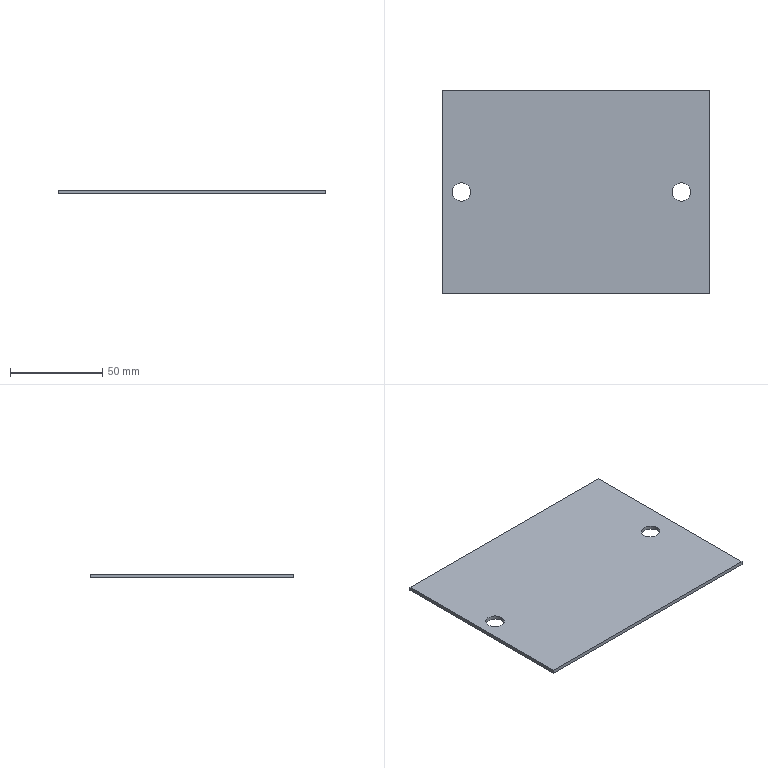Part | STEP file | 1 solid | 10 faces | box 144 x 110 x 2 mm | volume 31366 mm3 | plane 6 | cylinder 4 | commonest cylinder face diameters 10 x4
STEP:
#1=CARTESIAN_POINT('',(0.,0.,0.));
#2=DIRECTION('',(0.,0.,1.));
#3=DIRECTION('',(1.,0.,0.));
#4=AXIS2_PLACEMENT_3D('',#1,#2,#3);
#5=CARTESIAN_POINT('',(31.918,33.653,2.));
#6=VERTEX_POINT('',#5);
#7=CARTESIAN_POINT('',(31.918,33.653,0.));
#8=VERTEX_POINT('',#7);
#9=CARTESIAN_POINT('',(31.918,33.653,2.));
#10=DIRECTION('',(0.,0.,-1.));
#11=VECTOR('',#10,1.);
#12=LINE('',#9,#11);
#13=CARTESIAN_POINT('',(36.918,33.653,2.));
#14=DIRECTION('',(0.,0.,-1.));
#15=DIRECTION('',(-1.,0.,0.));
#16=AXIS2_PLACEMENT_3D('',#13,#14,#15);
#17=CYLINDRICAL_SURFACE('',#16,5.);
#18=CARTESIAN_POINT('',(6.283,0.));
#19=DIRECTION('',(0.,1.));
#20=VECTOR('',#19,1.);
#21=LINE('',#18,#20);
#22=(GEOMETRIC_REPRESENTATION_CONTEXT(2)PARAMETRIC_REPRESENTATION_CONTEXT()REPRESENTATION_CONTEXT('',''));
#23=DEFINITIONAL_REPRESENTATION('',(#21),#22);
#24=PCURVE('',#17,#23);
#25=CARTESIAN_POINT('',(36.918,33.653,2.));
#26=DIRECTION('',(0.,0.,-1.));
#27=DIRECTION('',(-1.,0.,0.));
#28=AXIS2_PLACEMENT_3D('',#25,#26,#27);
#29=CYLINDRICAL_SURFACE('',#28,5.);
#30=CARTESIAN_POINT('',(0.,0.));
#31=DIRECTION('',(0.,1.));
#32=VECTOR('',#31,1.);
#33=LINE('',#30,#32);
#34=(GEOMETRIC_REPRESENTATION_CONTEXT(2)PARAMETRIC_REPRESENTATION_CONTEXT()REPRESENTATION_CONTEXT('',''));
#35=DEFINITIONAL_REPRESENTATION('',(#33),#34);
#36=PCURVE('',#29,#35);
#37=SURFACE_CURVE('',#12,(#24,#36),.PCURVE_S1.);
#38=EDGE_CURVE('',#6,#8,#37,.T.);
#39=ORIENTED_EDGE('',*,*,#38,.T.);
#40=CARTESIAN_POINT('',(41.918,33.653,0.));
#41=VERTEX_POINT('',#40);
#42=CARTESIAN_POINT('',(36.918,33.653,0.));
#43=DIRECTION('',(0.,0.,-1.));
#44=DIRECTION('',(-1.,0.,0.));
#45=AXIS2_PLACEMENT_3D('',#42,#43,#44);
#46=CIRCLE('',#45,5.);
#47=CARTESIAN_POINT('',(0.,2.));
#48=DIRECTION('',(1.,0.));
#49=VECTOR('',#48,1.);
#50=LINE('',#47,#49);
#51=(GEOMETRIC_REPRESENTATION_CONTEXT(2)PARAMETRIC_REPRESENTATION_CONTEXT()REPRESENTATION_CONTEXT('',''));
#52=DEFINITIONAL_REPRESENTATION('',(#50),#51);
#53=PCURVE('',#17,#52);
#54=CARTESIAN_POINT('',(-20.082,33.653,0.));
#55=DIRECTION('',(0.,0.,1.));
#56=DIRECTION('',(1.,0.,0.));
#57=AXIS2_PLACEMENT_3D('',#54,#55,#56);
#58=PLANE('',#57);
#59=CARTESIAN_POINT('',(52.,0.));
#60=CARTESIAN_POINT('',(52.,8.66));
#61=CARTESIAN_POINT('',(59.5,4.33));
#62=CARTESIAN_POINT('',(67.,0.));
#63=CARTESIAN_POINT('',(59.5,-4.33));
#64=CARTESIAN_POINT('',(52.,-8.66));
#65=CARTESIAN_POINT('',(52.,0.));
#66=(BOUNDED_CURVE()B_SPLINE_CURVE(2,(#59,#60,#61,#62,#63,#64,#65),.UNSPECIFIED.,.T.,.F.)B_SPLINE_CURVE_WITH_KNOTS((1,2,2,2,2,1),(-2.094,0.,2.094,4.189,6.283,8.378),.UNSPECIFIED.)CURVE()GEOMETRIC_REPRESENTATION_ITEM()RATIONAL_B_SPLINE_CURVE((1.,0.5,1.,0.5,1.,0.5,1.))REPRESENTATION_ITEM(''));
#67=(GEOMETRIC_REPRESENTATION_CONTEXT(2)PARAMETRIC_REPRESENTATION_CONTEXT()REPRESENTATION_CONTEXT('',''));
#68=DEFINITIONAL_REPRESENTATION('',(#66),#67);
#69=PCURVE('',#58,#68);
#70=SURFACE_CURVE('',#46,(#53,#69),.PCURVE_S1.);
#71=EDGE_CURVE('',#41,#8,#70,.T.);
#72=ORIENTED_EDGE('',*,*,#71,.F.);
#73=CARTESIAN_POINT('',(41.918,33.653,2.));
#74=VERTEX_POINT('',#73);
#75=CARTESIAN_POINT('',(41.918,33.653,2.));
#76=DIRECTION('',(0.,0.,-1.));
#77=VECTOR('',#76,1.);
#78=LINE('',#75,#77);
#79=CARTESIAN_POINT('',(3.142,0.));
#80=DIRECTION('',(0.,1.));
#81=VECTOR('',#80,1.);
#82=LINE('',#79,#81);
#83=(GEOMETRIC_REPRESENTATION_CONTEXT(2)PARAMETRIC_REPRESENTATION_CONTEXT()REPRESENTATION_CONTEXT('',''));
#84=DEFINITIONAL_REPRESENTATION('',(#82),#83);
#85=PCURVE('',#17,#84);
#86=CARTESIAN_POINT('',(3.142,0.));
#87=DIRECTION('',(0.,1.));
#88=VECTOR('',#87,1.);
#89=LINE('',#86,#88);
#90=(GEOMETRIC_REPRESENTATION_CONTEXT(2)PARAMETRIC_REPRESENTATION_CONTEXT()REPRESENTATION_CONTEXT('',''));
#91=DEFINITIONAL_REPRESENTATION('',(#89),#90);
#92=PCURVE('',#29,#91);
#93=SURFACE_CURVE('',#78,(#85,#92),.PCURVE_S1.);
#94=EDGE_CURVE('',#74,#41,#93,.T.);
#95=ORIENTED_EDGE('',*,*,#94,.F.);
#96=CARTESIAN_POINT('',(36.918,33.653,2.));
#97=DIRECTION('',(0.,0.,-1.));
#98=DIRECTION('',(-1.,0.,0.));
#99=AXIS2_PLACEMENT_3D('',#96,#97,#98);
#100=CIRCLE('',#99,5.);
#101=CARTESIAN_POINT('',(0.,0.));
#102=DIRECTION('',(1.,0.));
#103=VECTOR('',#102,1.);
#104=LINE('',#101,#103);
#105=(GEOMETRIC_REPRESENTATION_CONTEXT(2)PARAMETRIC_REPRESENTATION_CONTEXT()REPRESENTATION_CONTEXT('',''));
#106=DEFINITIONAL_REPRESENTATION('',(#104),#105);
#107=PCURVE('',#17,#106);
#108=CARTESIAN_POINT('',(-20.082,33.653,2.));
#109=DIRECTION('',(0.,0.,1.));
#110=DIRECTION('',(1.,0.,0.));
#111=AXIS2_PLACEMENT_3D('',#108,#109,#110);
#112=PLANE('',#111);
#113=CARTESIAN_POINT('',(52.,0.));
#114=CARTESIAN_POINT('',(52.,8.66));
#115=CARTESIAN_POINT('',(59.5,4.33));
#116=CARTESIAN_POINT('',(67.,0.));
#117=CARTESIAN_POINT('',(59.5,-4.33));
#118=CARTESIAN_POINT('',(52.,-8.66));
#119=CARTESIAN_POINT('',(52.,0.));
#120=(BOUNDED_CURVE()B_SPLINE_CURVE(2,(#113,#114,#115,#116,#117,#118,#119),.UNSPECIFIED.,.T.,.F.)B_SPLINE_CURVE_WITH_KNOTS((1,2,2,2,2,1),(-2.094,0.,2.094,4.189,6.283,8.378),.UNSPECIFIED.)CURVE()GEOMETRIC_REPRESENTATION_ITEM()RATIONAL_B_SPLINE_CURVE((1.,0.5,1.,0.5,1.,0.5,1.))REPRESENTATION_ITEM(''));
#121=(GEOMETRIC_REPRESENTATION_CONTEXT(2)PARAMETRIC_REPRESENTATION_CONTEXT()REPRESENTATION_CONTEXT('',''));
#122=DEFINITIONAL_REPRESENTATION('',(#120),#121);
#123=PCURVE('',#112,#122);
#124=SURFACE_CURVE('',#100,(#107,#123),.PCURVE_S1.);
#125=EDGE_CURVE('',#74,#6,#124,.T.);
#126=ORIENTED_EDGE('',*,*,#125,.T.);
#127=EDGE_LOOP('',(#39,#72,#95,#126));
#128=FACE_BOUND('',#127,.F.);
#129=ADVANCED_FACE('',(#128),#17,.F.);
#130=CARTESIAN_POINT('',(-87.082,33.653,2.));
#131=VERTEX_POINT('',#130);
#132=CARTESIAN_POINT('',(-87.082,33.653,0.));
#133=VERTEX_POINT('',#132);
#134=CARTESIAN_POINT('',(-87.082,33.653,2.));
#135=DIRECTION('',(0.,0.,-1.));
#136=VECTOR('',#135,1.);
#137=LINE('',#134,#136);
#138=CARTESIAN_POINT('',(-82.082,33.653,2.));
#139=DIRECTION('',(0.,0.,-1.));
#140=DIRECTION('',(-1.,0.,0.));
#141=AXIS2_PLACEMENT_3D('',#138,#139,#140);
#142=CYLINDRICAL_SURFACE('',#141,5.);
#143=CARTESIAN_POINT('',(6.283,0.));
#144=DIRECTION('',(0.,1.));
#145=VECTOR('',#144,1.);
#146=LINE('',#143,#145);
#147=(GEOMETRIC_REPRESENTATION_CONTEXT(2)PARAMETRIC_REPRESENTATION_CONTEXT()REPRESENTATION_CONTEXT('',''));
#148=DEFINITIONAL_REPRESENTATION('',(#146),#147);
#149=PCURVE('',#142,#148);
#150=CARTESIAN_POINT('',(-82.082,33.653,2.));
#151=DIRECTION('',(0.,0.,-1.));
#152=DIRECTION('',(-1.,0.,0.));
#153=AXIS2_PLACEMENT_3D('',#150,#151,#152);
#154=CYLINDRICAL_SURFACE('',#153,5.);
#155=CARTESIAN_POINT('',(0.,0.));
#156=DIRECTION('',(0.,1.));
#157=VECTOR('',#156,1.);
#158=LINE('',#155,#157);
#159=(GEOMETRIC_REPRESENTATION_CONTEXT(2)PARAMETRIC_REPRESENTATION_CONTEXT()REPRESENTATION_CONTEXT('',''));
#160=DEFINITIONAL_REPRESENTATION('',(#158),#159);
#161=PCURVE('',#154,#160);
#162=SURFACE_CURVE('',#137,(#149,#161),.PCURVE_S1.);
#163=EDGE_CURVE('',#131,#133,#162,.T.);
#164=ORIENTED_EDGE('',*,*,#163,.T.);
#165=CARTESIAN_POINT('',(-77.082,33.653,0.));
#166=VERTEX_POINT('',#165);
#167=CARTESIAN_POINT('',(-82.082,33.653,0.));
#168=DIRECTION('',(0.,0.,-1.));
#169=DIRECTION('',(-1.,0.,0.));
#170=AXIS2_PLACEMENT_3D('',#167,#168,#169);
#171=CIRCLE('',#170,5.);
#172=CARTESIAN_POINT('',(0.,2.));
#173=DIRECTION('',(1.,0.));
#174=VECTOR('',#173,1.);
#175=LINE('',#172,#174);
#176=(GEOMETRIC_REPRESENTATION_CONTEXT(2)PARAMETRIC_REPRESENTATION_CONTEXT()REPRESENTATION_CONTEXT('',''));
#177=DEFINITIONAL_REPRESENTATION('',(#175),#176);
#178=PCURVE('',#142,#177);
#179=CARTESIAN_POINT('',(-67.,0.));
#180=CARTESIAN_POINT('',(-67.,8.66));
#181=CARTESIAN_POINT('',(-59.5,4.33));
#182=CARTESIAN_POINT('',(-52.,0.));
#183=CARTESIAN_POINT('',(-59.5,-4.33));
#184=CARTESIAN_POINT('',(-67.,-8.66));
#185=CARTESIAN_POINT('',(-67.,0.));
#186=(BOUNDED_CURVE()B_SPLINE_CURVE(2,(#179,#180,#181,#182,#183,#184,#185),.UNSPECIFIED.,.T.,.F.)B_SPLINE_CURVE_WITH_KNOTS((1,2,2,2,2,1),(-2.094,0.,2.094,4.189,6.283,8.378),.UNSPECIFIED.)CURVE()GEOMETRIC_REPRESENTATION_ITEM()RATIONAL_B_SPLINE_CURVE((1.,0.5,1.,0.5,1.,0.5,1.))REPRESENTATION_ITEM(''));
#187=(GEOMETRIC_REPRESENTATION_CONTEXT(2)PARAMETRIC_REPRESENTATION_CONTEXT()REPRESENTATION_CONTEXT('',''));
#188=DEFINITIONAL_REPRESENTATION('',(#186),#187);
#189=PCURVE('',#58,#188);
#190=SURFACE_CURVE('',#171,(#178,#189),.PCURVE_S1.);
#191=EDGE_CURVE('',#166,#133,#190,.T.);
#192=ORIENTED_EDGE('',*,*,#191,.F.);
#193=CARTESIAN_POINT('',(-77.082,33.653,2.));
#194=VERTEX_POINT('',#193);
#195=CARTESIAN_POINT('',(-77.082,33.653,2.));
#196=DIRECTION('',(0.,0.,-1.));
#197=VECTOR('',#196,1.);
#198=LINE('',#195,#197);
#199=CARTESIAN_POINT('',(3.142,0.));
#200=DIRECTION('',(0.,1.));
#201=VECTOR('',#200,1.);
#202=LINE('',#199,#201);
#203=(GEOMETRIC_REPRESENTATION_CONTEXT(2)PARAMETRIC_REPRESENTATION_CONTEXT()REPRESENTATION_CONTEXT('',''));
#204=DEFINITIONAL_REPRESENTATION('',(#202),#203);
#205=PCURVE('',#142,#204);
#206=CARTESIAN_POINT('',(3.142,0.));
#207=DIRECTION('',(0.,1.));
#208=VECTOR('',#207,1.);
#209=LINE('',#206,#208);
#210=(GEOMETRIC_REPRESENTATION_CONTEXT(2)PARAMETRIC_REPRESENTATION_CONTEXT()REPRESENTATION_CONTEXT('',''));
#211=DEFINITIONAL_REPRESENTATION('',(#209),#210);
#212=PCURVE('',#154,#211);
#213=SURFACE_CURVE('',#198,(#205,#212),.PCURVE_S1.);
#214=EDGE_CURVE('',#194,#166,#213,.T.);
#215=ORIENTED_EDGE('',*,*,#214,.F.);
#216=CARTESIAN_POINT('',(-82.082,33.653,2.));
#217=DIRECTION('',(0.,0.,-1.));
#218=DIRECTION('',(-1.,0.,0.));
#219=AXIS2_PLACEMENT_3D('',#216,#217,#218);
#220=CIRCLE('',#219,5.);
#221=CARTESIAN_POINT('',(0.,0.));
#222=DIRECTION('',(1.,0.));
#223=VECTOR('',#222,1.);
#224=LINE('',#221,#223);
#225=(GEOMETRIC_REPRESENTATION_CONTEXT(2)PARAMETRIC_REPRESENTATION_CONTEXT()REPRESENTATION_CONTEXT('',''));
#226=DEFINITIONAL_REPRESENTATION('',(#224),#225);
#227=PCURVE('',#142,#226);
#228=CARTESIAN_POINT('',(-67.,0.));
#229=CARTESIAN_POINT('',(-67.,8.66));
#230=CARTESIAN_POINT('',(-59.5,4.33));
#231=CARTESIAN_POINT('',(-52.,0.));
#232=CARTESIAN_POINT('',(-59.5,-4.33));
#233=CARTESIAN_POINT('',(-67.,-8.66));
#234=CARTESIAN_POINT('',(-67.,0.));
#235=(BOUNDED_CURVE()B_SPLINE_CURVE(2,(#228,#229,#230,#231,#232,#233,#234),.UNSPECIFIED.,.T.,.F.)B_SPLINE_CURVE_WITH_KNOTS((1,2,2,2,2,1),(-2.094,0.,2.094,4.189,6.283,8.378),.UNSPECIFIED.)CURVE()GEOMETRIC_REPRESENTATION_ITEM()RATIONAL_B_SPLINE_CURVE((1.,0.5,1.,0.5,1.,0.5,1.))REPRESENTATION_ITEM(''));
#236=(GEOMETRIC_REPRESENTATION_CONTEXT(2)PARAMETRIC_REPRESENTATION_CONTEXT()REPRESENTATION_CONTEXT('',''));
#237=DEFINITIONAL_REPRESENTATION('',(#235),#236);
#238=PCURVE('',#112,#237);
#239=SURFACE_CURVE('',#220,(#227,#238),.PCURVE_S1.);
#240=EDGE_CURVE('',#194,#131,#239,.T.);
#241=ORIENTED_EDGE('',*,*,#240,.T.);
#242=EDGE_LOOP('',(#164,#192,#215,#241));
#243=FACE_BOUND('',#242,.F.);
#244=ADVANCED_FACE('',(#243),#142,.F.);
#245=CARTESIAN_POINT('',(51.918,-21.347,0.));
#246=VERTEX_POINT('',#245);
#247=CARTESIAN_POINT('',(51.918,88.653,0.));
#248=VERTEX_POINT('',#247);
#249=CARTESIAN_POINT('',(51.918,33.653,0.));
#250=DIRECTION('',(0.,1.,0.));
#251=VECTOR('',#250,1.);
#252=LINE('',#249,#251);
#253=CARTESIAN_POINT('',(72.,0.));
#254=DIRECTION('',(0.,1.));
#255=VECTOR('',#254,1.);
#256=LINE('',#253,#255);
#257=(GEOMETRIC_REPRESENTATION_CONTEXT(2)PARAMETRIC_REPRESENTATION_CONTEXT()REPRESENTATION_CONTEXT('',''));
#258=DEFINITIONAL_REPRESENTATION('',(#256),#257);
#259=PCURVE('',#58,#258);
#260=CARTESIAN_POINT('',(51.918,-21.347,0.));
#261=DIRECTION('',(1.,0.,0.));
#262=DIRECTION('',(0.,1.,0.));
#263=AXIS2_PLACEMENT_3D('',#260,#261,#262);
#264=PLANE('',#263);
#265=CARTESIAN_POINT('',(55.,0.));
#266=DIRECTION('',(1.,0.));
#267=VECTOR('',#266,1.);
#268=LINE('',#265,#267);
#269=(GEOMETRIC_REPRESENTATION_CONTEXT(2)PARAMETRIC_REPRESENTATION_CONTEXT()REPRESENTATION_CONTEXT('',''));
#270=DEFINITIONAL_REPRESENTATION('',(#268),#269);
#271=PCURVE('',#264,#270);
#272=SURFACE_CURVE('',#252,(#259,#271),.PCURVE_S1.);
#273=EDGE_CURVE('',#246,#248,#272,.T.);
#274=ORIENTED_EDGE('',*,*,#273,.F.);
#275=CARTESIAN_POINT('',(-92.082,-21.347,0.));
#276=VERTEX_POINT('',#275);
#277=CARTESIAN_POINT('',(-20.082,-21.347,0.));
#278=DIRECTION('',(1.,0.,0.));
#279=VECTOR('',#278,1.);
#280=LINE('',#277,#279);
#281=CARTESIAN_POINT('',(0.,-55.));
#282=DIRECTION('',(1.,0.));
#283=VECTOR('',#282,1.);
#284=LINE('',#281,#283);
#285=(GEOMETRIC_REPRESENTATION_CONTEXT(2)PARAMETRIC_REPRESENTATION_CONTEXT()REPRESENTATION_CONTEXT('',''));
#286=DEFINITIONAL_REPRESENTATION('',(#284),#285);
#287=PCURVE('',#58,#286);
#288=CARTESIAN_POINT('',(-92.082,-21.347,0.));
#289=DIRECTION('',(0.,-1.,0.));
#290=DIRECTION('',(1.,0.,0.));
#291=AXIS2_PLACEMENT_3D('',#288,#289,#290);
#292=PLANE('',#291);
#293=CARTESIAN_POINT('',(72.,0.));
#294=DIRECTION('',(1.,0.));
#295=VECTOR('',#294,1.);
#296=LINE('',#293,#295);
#297=(GEOMETRIC_REPRESENTATION_CONTEXT(2)PARAMETRIC_REPRESENTATION_CONTEXT()REPRESENTATION_CONTEXT('',''));
#298=DEFINITIONAL_REPRESENTATION('',(#296),#297);
#299=PCURVE('',#292,#298);
#300=SURFACE_CURVE('',#280,(#287,#299),.PCURVE_S1.);
#301=EDGE_CURVE('',#276,#246,#300,.T.);
#302=ORIENTED_EDGE('',*,*,#301,.F.);
#303=CARTESIAN_POINT('',(-92.082,88.653,0.));
#304=VERTEX_POINT('',#303);
#305=CARTESIAN_POINT('',(-92.082,33.653,0.));
#306=DIRECTION('',(0.,-1.,0.));
#307=VECTOR('',#306,1.);
#308=LINE('',#305,#307);
#309=CARTESIAN_POINT('',(-72.,0.));
#310=DIRECTION('',(0.,-1.));
#311=VECTOR('',#310,1.);
#312=LINE('',#309,#311);
#313=(GEOMETRIC_REPRESENTATION_CONTEXT(2)PARAMETRIC_REPRESENTATION_CONTEXT()REPRESENTATION_CONTEXT('',''));
#314=DEFINITIONAL_REPRESENTATION('',(#312),#313);
#315=PCURVE('',#58,#314);
#316=CARTESIAN_POINT('',(-92.082,88.653,0.));
#317=DIRECTION('',(-1.,0.,0.));
#318=DIRECTION('',(0.,-1.,0.));
#319=AXIS2_PLACEMENT_3D('',#316,#317,#318);
#320=PLANE('',#319);
#321=CARTESIAN_POINT('',(55.,0.));
#322=DIRECTION('',(1.,0.));
#323=VECTOR('',#322,1.);
#324=LINE('',#321,#323);
#325=(GEOMETRIC_REPRESENTATION_CONTEXT(2)PARAMETRIC_REPRESENTATION_CONTEXT()REPRESENTATION_CONTEXT('',''));
#326=DEFINITIONAL_REPRESENTATION('',(#324),#325);
#327=PCURVE('',#320,#326);
#328=SURFACE_CURVE('',#308,(#315,#327),.PCURVE_S1.);
#329=EDGE_CURVE('',#304,#276,#328,.T.);
#330=ORIENTED_EDGE('',*,*,#329,.F.);
#331=CARTESIAN_POINT('',(-20.082,88.653,0.));
#332=DIRECTION('',(-1.,0.,0.));
#333=VECTOR('',#332,1.);
#334=LINE('',#331,#333);
#335=CARTESIAN_POINT('',(0.,55.));
#336=DIRECTION('',(-1.,0.));
#337=VECTOR('',#336,1.);
#338=LINE('',#335,#337);
#339=(GEOMETRIC_REPRESENTATION_CONTEXT(2)PARAMETRIC_REPRESENTATION_CONTEXT()REPRESENTATION_CONTEXT('',''));
#340=DEFINITIONAL_REPRESENTATION('',(#338),#339);
#341=PCURVE('',#58,#340);
#342=CARTESIAN_POINT('',(51.918,88.653,0.));
#343=DIRECTION('',(0.,1.,0.));
#344=DIRECTION('',(0.,0.,1.));
#345=AXIS2_PLACEMENT_3D('',#342,#343,#344);
#346=PLANE('',#345);
#347=CARTESIAN_POINT('',(0.,-72.));
#348=DIRECTION('',(0.,-1.));
#349=VECTOR('',#348,1.);
#350=LINE('',#347,#349);
#351=(GEOMETRIC_REPRESENTATION_CONTEXT(2)PARAMETRIC_REPRESENTATION_CONTEXT()REPRESENTATION_CONTEXT('',''));
#352=DEFINITIONAL_REPRESENTATION('',(#350),#351);
#353=PCURVE('',#346,#352);
#354=SURFACE_CURVE('',#334,(#341,#353),.PCURVE_S1.);
#355=EDGE_CURVE('',#248,#304,#354,.T.);
#356=ORIENTED_EDGE('',*,*,#355,.F.);
#357=EDGE_LOOP('',(#274,#302,#330,#356));
#358=FACE_BOUND('',#357,.T.);
#359=CARTESIAN_POINT('',(36.918,33.653,0.));
#360=DIRECTION('',(0.,0.,-1.));
#361=DIRECTION('',(-1.,0.,0.));
#362=AXIS2_PLACEMENT_3D('',#359,#360,#361);
#363=CIRCLE('',#362,5.);
#364=CARTESIAN_POINT('',(52.,0.));
#365=CARTESIAN_POINT('',(52.,8.66));
#366=CARTESIAN_POINT('',(59.5,4.33));
#367=CARTESIAN_POINT('',(67.,0.));
#368=CARTESIAN_POINT('',(59.5,-4.33));
#369=CARTESIAN_POINT('',(52.,-8.66));
#370=CARTESIAN_POINT('',(52.,0.));
#371=(BOUNDED_CURVE()B_SPLINE_CURVE(2,(#364,#365,#366,#367,#368,#369,#370),.UNSPECIFIED.,.T.,.F.)B_SPLINE_CURVE_WITH_KNOTS((1,2,2,2,2,1),(-2.094,0.,2.094,4.189,6.283,8.378),.UNSPECIFIED.)CURVE()GEOMETRIC_REPRESENTATION_ITEM()RATIONAL_B_SPLINE_CURVE((1.,0.5,1.,0.5,1.,0.5,1.))REPRESENTATION_ITEM(''));
#372=(GEOMETRIC_REPRESENTATION_CONTEXT(2)PARAMETRIC_REPRESENTATION_CONTEXT()REPRESENTATION_CONTEXT('',''));
#373=DEFINITIONAL_REPRESENTATION('',(#371),#372);
#374=PCURVE('',#58,#373);
#375=CARTESIAN_POINT('',(0.,2.));
#376=DIRECTION('',(1.,0.));
#377=VECTOR('',#376,1.);
#378=LINE('',#375,#377);
#379=(GEOMETRIC_REPRESENTATION_CONTEXT(2)PARAMETRIC_REPRESENTATION_CONTEXT()REPRESENTATION_CONTEXT('',''));
#380=DEFINITIONAL_REPRESENTATION('',(#378),#379);
#381=PCURVE('',#29,#380);
#382=SURFACE_CURVE('',#363,(#374,#381),.PCURVE_S1.);
#383=EDGE_CURVE('',#8,#41,#382,.T.);
#384=ORIENTED_EDGE('',*,*,#383,.F.);
#385=ORIENTED_EDGE('',*,*,#71,.F.);
#386=EDGE_LOOP('',(#384,#385));
#387=FACE_BOUND('',#386,.T.);
#388=CARTESIAN_POINT('',(-82.082,33.653,0.));
#389=DIRECTION('',(0.,0.,-1.));
#390=DIRECTION('',(-1.,0.,0.));
#391=AXIS2_PLACEMENT_3D('',#388,#389,#390);
#392=CIRCLE('',#391,5.);
#393=CARTESIAN_POINT('',(-67.,0.));
#394=CARTESIAN_POINT('',(-67.,8.66));
#395=CARTESIAN_POINT('',(-59.5,4.33));
#396=CARTESIAN_POINT('',(-52.,0.));
#397=CARTESIAN_POINT('',(-59.5,-4.33));
#398=CARTESIAN_POINT('',(-67.,-8.66));
#399=CARTESIAN_POINT('',(-67.,0.));
#400=(BOUNDED_CURVE()B_SPLINE_CURVE(2,(#393,#394,#395,#396,#397,#398,#399),.UNSPECIFIED.,.T.,.F.)B_SPLINE_CURVE_WITH_KNOTS((1,2,2,2,2,1),(-2.094,0.,2.094,4.189,6.283,8.378),.UNSPECIFIED.)CURVE()GEOMETRIC_REPRESENTATION_ITEM()RATIONAL_B_SPLINE_CURVE((1.,0.5,1.,0.5,1.,0.5,1.))REPRESENTATION_ITEM(''));
#401=(GEOMETRIC_REPRESENTATION_CONTEXT(2)PARAMETRIC_REPRESENTATION_CONTEXT()REPRESENTATION_CONTEXT('',''));
#402=DEFINITIONAL_REPRESENTATION('',(#400),#401);
#403=PCURVE('',#58,#402);
#404=CARTESIAN_POINT('',(0.,2.));
#405=DIRECTION('',(1.,0.));
#406=VECTOR('',#405,1.);
#407=LINE('',#404,#406);
#408=(GEOMETRIC_REPRESENTATION_CONTEXT(2)PARAMETRIC_REPRESENTATION_CONTEXT()REPRESENTATION_CONTEXT('',''));
#409=DEFINITIONAL_REPRESENTATION('',(#407),#408);
#410=PCURVE('',#154,#409);
#411=SURFACE_CURVE('',#392,(#403,#410),.PCURVE_S1.);
#412=EDGE_CURVE('',#133,#166,#411,.T.);
#413=ORIENTED_EDGE('',*,*,#412,.F.);
#414=ORIENTED_EDGE('',*,*,#191,.F.);
#415=EDGE_LOOP('',(#413,#414));
#416=FACE_BOUND('',#415,.T.);
#417=ADVANCED_FACE('',(#358,#387,#416),#58,.F.);
#418=CARTESIAN_POINT('',(-92.082,88.653,2.));
#419=VERTEX_POINT('',#418);
#420=CARTESIAN_POINT('',(51.918,88.653,2.));
#421=VERTEX_POINT('',#420);
#422=CARTESIAN_POINT('',(51.918,88.653,2.));
#423=DIRECTION('',(1.,0.,0.));
#424=VECTOR('',#423,1.);
#425=LINE('',#422,#424);
#426=CARTESIAN_POINT('',(2.,0.));
#427=DIRECTION('',(0.,1.));
#428=VECTOR('',#427,1.);
#429=LINE('',#426,#428);
#430=(GEOMETRIC_REPRESENTATION_CONTEXT(2)PARAMETRIC_REPRESENTATION_CONTEXT()REPRESENTATION_CONTEXT('',''));
#431=DEFINITIONAL_REPRESENTATION('',(#429),#430);
#432=PCURVE('',#346,#431);
#433=CARTESIAN_POINT('',(72.,55.));
#434=DIRECTION('',(1.,0.));
#435=VECTOR('',#434,1.);
#436=LINE('',#433,#435);
#437=(GEOMETRIC_REPRESENTATION_CONTEXT(2)PARAMETRIC_REPRESENTATION_CONTEXT()REPRESENTATION_CONTEXT('',''));
#438=DEFINITIONAL_REPRESENTATION('',(#436),#437);
#439=PCURVE('',#112,#438);
#440=SURFACE_CURVE('',#425,(#432,#439),.PCURVE_S1.);
#441=EDGE_CURVE('',#419,#421,#440,.T.);
#442=ORIENTED_EDGE('',*,*,#441,.T.);
#443=CARTESIAN_POINT('',(51.918,88.653,0.));
#444=DIRECTION('',(0.,0.,-1.));
#445=VECTOR('',#444,1.);
#446=LINE('',#443,#445);
#447=CARTESIAN_POINT('',(0.,0.));
#448=DIRECTION('',(-1.,0.));
#449=VECTOR('',#448,1.);
#450=LINE('',#447,#449);
#451=(GEOMETRIC_REPRESENTATION_CONTEXT(2)PARAMETRIC_REPRESENTATION_CONTEXT()REPRESENTATION_CONTEXT('',''));
#452=DEFINITIONAL_REPRESENTATION('',(#450),#451);
#453=PCURVE('',#346,#452);
#454=CARTESIAN_POINT('',(110.,0.));
#455=DIRECTION('',(0.,-1.));
#456=VECTOR('',#455,1.);
#457=LINE('',#454,#456);
#458=(GEOMETRIC_REPRESENTATION_CONTEXT(2)PARAMETRIC_REPRESENTATION_CONTEXT()REPRESENTATION_CONTEXT('',''));
#459=DEFINITIONAL_REPRESENTATION('',(#457),#458);
#460=PCURVE('',#264,#459);
#461=SURFACE_CURVE('',#446,(#453,#460),.PCURVE_S1.);
#462=EDGE_CURVE('',#421,#248,#461,.T.);
#463=ORIENTED_EDGE('',*,*,#462,.T.);
#464=ORIENTED_EDGE('',*,*,#355,.T.);
#465=CARTESIAN_POINT('',(-92.082,88.653,0.));
#466=DIRECTION('',(0.,0.,1.));
#467=VECTOR('',#466,1.);
#468=LINE('',#465,#467);
#469=CARTESIAN_POINT('',(0.,-144.));
#470=DIRECTION('',(1.,0.));
#471=VECTOR('',#470,1.);
#472=LINE('',#469,#471);
#473=(GEOMETRIC_REPRESENTATION_CONTEXT(2)PARAMETRIC_REPRESENTATION_CONTEXT()REPRESENTATION_CONTEXT('',''));
#474=DEFINITIONAL_REPRESENTATION('',(#472),#473);
#475=PCURVE('',#346,#474);
#476=CARTESIAN_POINT('',(0.,0.));
#477=DIRECTION('',(0.,1.));
#478=VECTOR('',#477,1.);
#479=LINE('',#476,#478);
#480=(GEOMETRIC_REPRESENTATION_CONTEXT(2)PARAMETRIC_REPRESENTATION_CONTEXT()REPRESENTATION_CONTEXT('',''));
#481=DEFINITIONAL_REPRESENTATION('',(#479),#480);
#482=PCURVE('',#320,#481);
#483=SURFACE_CURVE('',#468,(#475,#482),.PCURVE_S1.);
#484=EDGE_CURVE('',#304,#419,#483,.T.);
#485=ORIENTED_EDGE('',*,*,#484,.T.);
#486=EDGE_LOOP('',(#442,#463,#464,#485));
#487=FACE_BOUND('',#486,.T.);
#488=ADVANCED_FACE('',(#487),#346,.T.);
#489=CARTESIAN_POINT('',(51.918,-21.347,2.));
#490=VERTEX_POINT('',#489);
#491=CARTESIAN_POINT('',(51.918,-21.347,2.));
#492=DIRECTION('',(0.,-1.,0.));
#493=VECTOR('',#492,1.);
#494=LINE('',#491,#493);
#495=CARTESIAN_POINT('',(0.,2.));
#496=DIRECTION('',(-1.,0.));
#497=VECTOR('',#496,1.);
#498=LINE('',#495,#497);
#499=(GEOMETRIC_REPRESENTATION_CONTEXT(2)PARAMETRIC_REPRESENTATION_CONTEXT()REPRESENTATION_CONTEXT('',''));
#500=DEFINITIONAL_REPRESENTATION('',(#498),#499);
#501=PCURVE('',#264,#500);
#502=CARTESIAN_POINT('',(72.,-55.));
#503=DIRECTION('',(0.,-1.));
#504=VECTOR('',#503,1.);
#505=LINE('',#502,#504);
#506=(GEOMETRIC_REPRESENTATION_CONTEXT(2)PARAMETRIC_REPRESENTATION_CONTEXT()REPRESENTATION_CONTEXT('',''));
#507=DEFINITIONAL_REPRESENTATION('',(#505),#506);
#508=PCURVE('',#112,#507);
#509=SURFACE_CURVE('',#494,(#501,#508),.PCURVE_S1.);
#510=EDGE_CURVE('',#421,#490,#509,.T.);
#511=ORIENTED_EDGE('',*,*,#510,.T.);
#512=CARTESIAN_POINT('',(51.918,-21.347,0.));
#513=DIRECTION('',(0.,0.,-1.));
#514=VECTOR('',#513,1.);
#515=LINE('',#512,#514);
#516=CARTESIAN_POINT('',(0.,0.));
#517=DIRECTION('',(0.,-1.));
#518=VECTOR('',#517,1.);
#519=LINE('',#516,#518);
#520=(GEOMETRIC_REPRESENTATION_CONTEXT(2)PARAMETRIC_REPRESENTATION_CONTEXT()REPRESENTATION_CONTEXT('',''));
#521=DEFINITIONAL_REPRESENTATION('',(#519),#520);
#522=PCURVE('',#264,#521);
#523=CARTESIAN_POINT('',(144.,0.));
#524=DIRECTION('',(0.,-1.));
#525=VECTOR('',#524,1.);
#526=LINE('',#523,#525);
#527=(GEOMETRIC_REPRESENTATION_CONTEXT(2)PARAMETRIC_REPRESENTATION_CONTEXT()REPRESENTATION_CONTEXT('',''));
#528=DEFINITIONAL_REPRESENTATION('',(#526),#527);
#529=PCURVE('',#292,#528);
#530=SURFACE_CURVE('',#515,(#522,#529),.PCURVE_S1.);
#531=EDGE_CURVE('',#490,#246,#530,.T.);
#532=ORIENTED_EDGE('',*,*,#531,.T.);
#533=ORIENTED_EDGE('',*,*,#273,.T.);
#534=ORIENTED_EDGE('',*,*,#462,.F.);
#535=EDGE_LOOP('',(#511,#532,#533,#534));
#536=FACE_BOUND('',#535,.T.);
#537=ADVANCED_FACE('',(#536),#264,.T.);
#538=CARTESIAN_POINT('',(-92.082,-21.347,2.));
#539=VERTEX_POINT('',#538);
#540=CARTESIAN_POINT('',(-92.082,-21.347,2.));
#541=DIRECTION('',(-1.,0.,0.));
#542=VECTOR('',#541,1.);
#543=LINE('',#540,#542);
#544=CARTESIAN_POINT('',(0.,2.));
#545=DIRECTION('',(-1.,0.));
#546=VECTOR('',#545,1.);
#547=LINE('',#544,#546);
#548=(GEOMETRIC_REPRESENTATION_CONTEXT(2)PARAMETRIC_REPRESENTATION_CONTEXT()REPRESENTATION_CONTEXT('',''));
#549=DEFINITIONAL_REPRESENTATION('',(#547),#548);
#550=PCURVE('',#292,#549);
#551=CARTESIAN_POINT('',(-72.,-55.));
#552=DIRECTION('',(-1.,0.));
#553=VECTOR('',#552,1.);
#554=LINE('',#551,#553);
#555=(GEOMETRIC_REPRESENTATION_CONTEXT(2)PARAMETRIC_REPRESENTATION_CONTEXT()REPRESENTATION_CONTEXT('',''));
#556=DEFINITIONAL_REPRESENTATION('',(#554),#555);
#557=PCURVE('',#112,#556);
#558=SURFACE_CURVE('',#543,(#550,#557),.PCURVE_S1.);
#559=EDGE_CURVE('',#490,#539,#558,.T.);
#560=ORIENTED_EDGE('',*,*,#559,.T.);
#561=CARTESIAN_POINT('',(-92.082,-21.347,0.));
#562=DIRECTION('',(0.,0.,-1.));
#563=VECTOR('',#562,1.);
#564=LINE('',#561,#563);
#565=CARTESIAN_POINT('',(0.,0.));
#566=DIRECTION('',(0.,-1.));
#567=VECTOR('',#566,1.);
#568=LINE('',#565,#567);
#569=(GEOMETRIC_REPRESENTATION_CONTEXT(2)PARAMETRIC_REPRESENTATION_CONTEXT()REPRESENTATION_CONTEXT('',''));
#570=DEFINITIONAL_REPRESENTATION('',(#568),#569);
#571=PCURVE('',#292,#570);
#572=CARTESIAN_POINT('',(110.,0.));
#573=DIRECTION('',(0.,-1.));
#574=VECTOR('',#573,1.);
#575=LINE('',#572,#574);
#576=(GEOMETRIC_REPRESENTATION_CONTEXT(2)PARAMETRIC_REPRESENTATION_CONTEXT()REPRESENTATION_CONTEXT('',''));
#577=DEFINITIONAL_REPRESENTATION('',(#575),#576);
#578=PCURVE('',#320,#577);
#579=SURFACE_CURVE('',#564,(#571,#578),.PCURVE_S1.);
#580=EDGE_CURVE('',#539,#276,#579,.T.);
#581=ORIENTED_EDGE('',*,*,#580,.T.);
#582=ORIENTED_EDGE('',*,*,#301,.T.);
#583=ORIENTED_EDGE('',*,*,#531,.F.);
#584=EDGE_LOOP('',(#560,#581,#582,#583));
#585=FACE_BOUND('',#584,.T.);
#586=ADVANCED_FACE('',(#585),#292,.T.);
#587=CARTESIAN_POINT('',(-92.082,88.653,2.));
#588=DIRECTION('',(0.,1.,0.));
#589=VECTOR('',#588,1.);
#590=LINE('',#587,#589);
#591=CARTESIAN_POINT('',(0.,2.));
#592=DIRECTION('',(-1.,0.));
#593=VECTOR('',#592,1.);
#594=LINE('',#591,#593);
#595=(GEOMETRIC_REPRESENTATION_CONTEXT(2)PARAMETRIC_REPRESENTATION_CONTEXT()REPRESENTATION_CONTEXT('',''));
#596=DEFINITIONAL_REPRESENTATION('',(#594),#595);
#597=PCURVE('',#320,#596);
#598=CARTESIAN_POINT('',(-72.,55.));
#599=DIRECTION('',(0.,1.));
#600=VECTOR('',#599,1.);
#601=LINE('',#598,#600);
#602=(GEOMETRIC_REPRESENTATION_CONTEXT(2)PARAMETRIC_REPRESENTATION_CONTEXT()REPRESENTATION_CONTEXT('',''));
#603=DEFINITIONAL_REPRESENTATION('',(#601),#602);
#604=PCURVE('',#112,#603);
#605=SURFACE_CURVE('',#590,(#597,#604),.PCURVE_S1.);
#606=EDGE_CURVE('',#539,#419,#605,.T.);
#607=ORIENTED_EDGE('',*,*,#606,.T.);
#608=ORIENTED_EDGE('',*,*,#484,.F.);
#609=ORIENTED_EDGE('',*,*,#329,.T.);
#610=ORIENTED_EDGE('',*,*,#580,.F.);
#611=EDGE_LOOP('',(#607,#608,#609,#610));
#612=FACE_BOUND('',#611,.T.);
#613=ADVANCED_FACE('',(#612),#320,.T.);
#614=ORIENTED_EDGE('',*,*,#383,.F.);
#615=ORIENTED_EDGE('',*,*,#38,.F.);
#616=CARTESIAN_POINT('',(36.918,33.653,2.));
#617=DIRECTION('',(0.,0.,-1.));
#618=DIRECTION('',(-1.,0.,0.));
#619=AXIS2_PLACEMENT_3D('',#616,#617,#618);
#620=CIRCLE('',#619,5.);
#621=CARTESIAN_POINT('',(0.,0.));
#622=DIRECTION('',(1.,0.));
#623=VECTOR('',#622,1.);
#624=LINE('',#621,#623);
#625=(GEOMETRIC_REPRESENTATION_CONTEXT(2)PARAMETRIC_REPRESENTATION_CONTEXT()REPRESENTATION_CONTEXT('',''));
#626=DEFINITIONAL_REPRESENTATION('',(#624),#625);
#627=PCURVE('',#29,#626);
#628=CARTESIAN_POINT('',(52.,0.));
#629=CARTESIAN_POINT('',(52.,8.66));
#630=CARTESIAN_POINT('',(59.5,4.33));
#631=CARTESIAN_POINT('',(67.,0.));
#632=CARTESIAN_POINT('',(59.5,-4.33));
#633=CARTESIAN_POINT('',(52.,-8.66));
#634=CARTESIAN_POINT('',(52.,0.));
#635=(BOUNDED_CURVE()B_SPLINE_CURVE(2,(#628,#629,#630,#631,#632,#633,#634),.UNSPECIFIED.,.T.,.F.)B_SPLINE_CURVE_WITH_KNOTS((1,2,2,2,2,1),(-2.094,0.,2.094,4.189,6.283,8.378),.UNSPECIFIED.)CURVE()GEOMETRIC_REPRESENTATION_ITEM()RATIONAL_B_SPLINE_CURVE((1.,0.5,1.,0.5,1.,0.5,1.))REPRESENTATION_ITEM(''));
#636=(GEOMETRIC_REPRESENTATION_CONTEXT(2)PARAMETRIC_REPRESENTATION_CONTEXT()REPRESENTATION_CONTEXT('',''));
#637=DEFINITIONAL_REPRESENTATION('',(#635),#636);
#638=PCURVE('',#112,#637);
#639=SURFACE_CURVE('',#620,(#627,#638),.PCURVE_S1.);
#640=EDGE_CURVE('',#6,#74,#639,.T.);
#641=ORIENTED_EDGE('',*,*,#640,.T.);
#642=ORIENTED_EDGE('',*,*,#94,.T.);
#643=EDGE_LOOP('',(#614,#615,#641,#642));
#644=FACE_BOUND('',#643,.F.);
#645=ADVANCED_FACE('',(#644),#29,.F.);
#646=ORIENTED_EDGE('',*,*,#412,.F.);
#647=ORIENTED_EDGE('',*,*,#163,.F.);
#648=CARTESIAN_POINT('',(-82.082,33.653,2.));
#649=DIRECTION('',(0.,0.,-1.));
#650=DIRECTION('',(-1.,0.,0.));
#651=AXIS2_PLACEMENT_3D('',#648,#649,#650);
#652=CIRCLE('',#651,5.);
#653=CARTESIAN_POINT('',(0.,0.));
#654=DIRECTION('',(1.,0.));
#655=VECTOR('',#654,1.);
#656=LINE('',#653,#655);
#657=(GEOMETRIC_REPRESENTATION_CONTEXT(2)PARAMETRIC_REPRESENTATION_CONTEXT()REPRESENTATION_CONTEXT('',''));
#658=DEFINITIONAL_REPRESENTATION('',(#656),#657);
#659=PCURVE('',#154,#658);
#660=CARTESIAN_POINT('',(-67.,0.));
#661=CARTESIAN_POINT('',(-67.,8.66));
#662=CARTESIAN_POINT('',(-59.5,4.33));
#663=CARTESIAN_POINT('',(-52.,0.));
#664=CARTESIAN_POINT('',(-59.5,-4.33));
#665=CARTESIAN_POINT('',(-67.,-8.66));
#666=CARTESIAN_POINT('',(-67.,0.));
#667=(BOUNDED_CURVE()B_SPLINE_CURVE(2,(#660,#661,#662,#663,#664,#665,#666),.UNSPECIFIED.,.T.,.F.)B_SPLINE_CURVE_WITH_KNOTS((1,2,2,2,2,1),(-2.094,0.,2.094,4.189,6.283,8.378),.UNSPECIFIED.)CURVE()GEOMETRIC_REPRESENTATION_ITEM()RATIONAL_B_SPLINE_CURVE((1.,0.5,1.,0.5,1.,0.5,1.))REPRESENTATION_ITEM(''));
#668=(GEOMETRIC_REPRESENTATION_CONTEXT(2)PARAMETRIC_REPRESENTATION_CONTEXT()REPRESENTATION_CONTEXT('',''));
#669=DEFINITIONAL_REPRESENTATION('',(#667),#668);
#670=PCURVE('',#112,#669);
#671=SURFACE_CURVE('',#652,(#659,#670),.PCURVE_S1.);
#672=EDGE_CURVE('',#131,#194,#671,.T.);
#673=ORIENTED_EDGE('',*,*,#672,.T.);
#674=ORIENTED_EDGE('',*,*,#214,.T.);
#675=EDGE_LOOP('',(#646,#647,#673,#674));
#676=FACE_BOUND('',#675,.F.);
#677=ADVANCED_FACE('',(#676),#154,.F.);
#678=ORIENTED_EDGE('',*,*,#559,.F.);
#679=ORIENTED_EDGE('',*,*,#510,.F.);
#680=ORIENTED_EDGE('',*,*,#441,.F.);
#681=ORIENTED_EDGE('',*,*,#606,.F.);
#682=EDGE_LOOP('',(#678,#679,#680,#681));
#683=FACE_BOUND('',#682,.T.);
#684=ORIENTED_EDGE('',*,*,#640,.T.);
#685=ORIENTED_EDGE('',*,*,#125,.T.);
#686=EDGE_LOOP('',(#684,#685));
#687=FACE_BOUND('',#686,.T.);
#688=ORIENTED_EDGE('',*,*,#672,.T.);
#689=ORIENTED_EDGE('',*,*,#240,.T.);
#690=EDGE_LOOP('',(#688,#689));
#691=FACE_BOUND('',#690,.T.);
#692=ADVANCED_FACE('',(#683,#687,#691),#112,.T.);
#693=CLOSED_SHELL('',(#129,#244,#417,#488,#537,#586,#613,#645,#677,#692));
#694=MANIFOLD_SOLID_BREP('',#693);
#695=(LENGTH_UNIT()NAMED_UNIT(*)SI_UNIT(.MILLI.,.METRE.));
#696=UNCERTAINTY_MEASURE_WITH_UNIT(LENGTH_MEASURE(0.0000001),#695,'','');
#697=(NAMED_UNIT(*)PLANE_ANGLE_UNIT()SI_UNIT($,.RADIAN.));
#698=(NAMED_UNIT(*)SI_UNIT($,.STERADIAN.)SOLID_ANGLE_UNIT());
#699=(GEOMETRIC_REPRESENTATION_CONTEXT(3)GLOBAL_UNCERTAINTY_ASSIGNED_CONTEXT((#696))GLOBAL_UNIT_ASSIGNED_CONTEXT((#695,#697,#698))REPRESENTATION_CONTEXT('',''));
#700=ADVANCED_BREP_SHAPE_REPRESENTATION('',(#4,#694),#699);